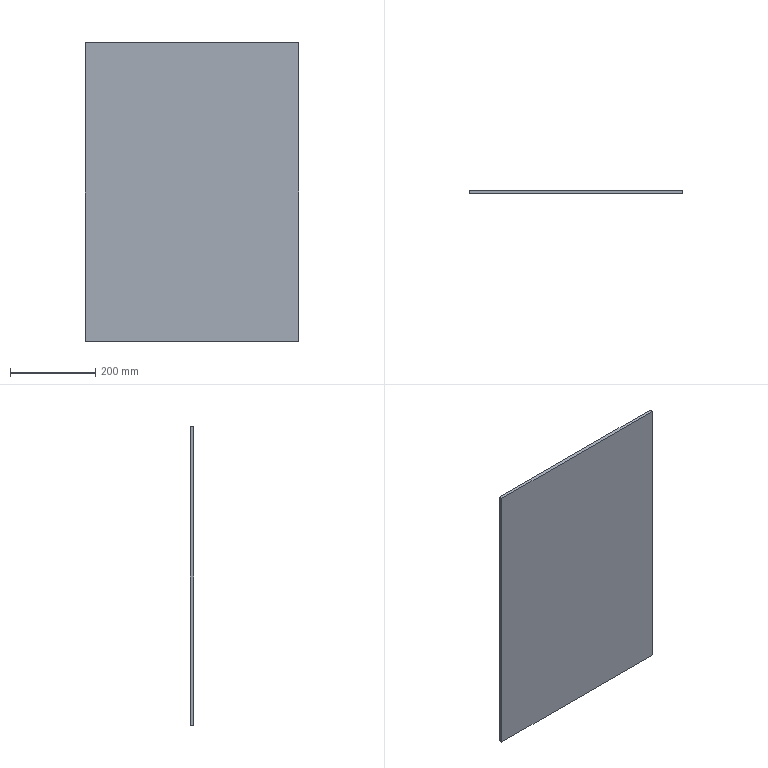Part | SolidWorks | features FlatPattern 1, SMBaseFlange 1, SheetMetal 1 | 1 solid | 6 faces | box 500 x 8 x 700 mm | volume 2800000 mm3 | plane 6
STEP:
#1=CARTESIAN_POINT('',(0.,0.,-700.));
#2=VERTEX_POINT('',#1);
#3=CARTESIAN_POINT('',(0.,0.,0.));
#4=VERTEX_POINT('',#3);
#5=CARTESIAN_POINT('',(0.,0.,0.));
#6=DIRECTION('',(0.,0.,1.));
#7=VECTOR('',#6,1000.);
#8=LINE('',#5,#7);
#9=EDGE_CURVE('',#2,#4,#8,.T.);
#10=ORIENTED_EDGE('',*,*,#9,.F.);
#11=CARTESIAN_POINT('',(0.,-8.,-700.));
#12=VERTEX_POINT('',#11);
#13=CARTESIAN_POINT('',(0.,-8.,-700.));
#14=DIRECTION('',(0.,1.,0.));
#15=VECTOR('',#14,1000.);
#16=LINE('',#13,#15);
#17=EDGE_CURVE('',#12,#2,#16,.T.);
#18=ORIENTED_EDGE('',*,*,#17,.F.);
#19=CARTESIAN_POINT('',(0.,-8.,0.));
#20=VERTEX_POINT('',#19);
#21=CARTESIAN_POINT('',(0.,-8.,0.));
#22=DIRECTION('',(0.,0.,1.));
#23=VECTOR('',#22,1000.);
#24=LINE('',#21,#23);
#25=EDGE_CURVE('',#12,#20,#24,.T.);
#26=ORIENTED_EDGE('',*,*,#25,.T.);
#27=CARTESIAN_POINT('',(0.,-8.,0.));
#28=DIRECTION('',(0.,1.,0.));
#29=VECTOR('',#28,1000.);
#30=LINE('',#27,#29);
#31=EDGE_CURVE('',#20,#4,#30,.T.);
#32=ORIENTED_EDGE('',*,*,#31,.T.);
#33=EDGE_LOOP('',(#10,#18,#26,#32));
#34=FACE_OUTER_BOUND('',#33,.T.);
#35=CARTESIAN_POINT('',(0.,-8.,0.));
#36=DIRECTION('',(-1.,0.,0.));
#37=DIRECTION('',(0.,0.,1.));
#38=AXIS2_PLACEMENT_3D('',#35,#36,#37);
#39=PLANE('',#38);
#40=ADVANCED_FACE('',(#34),#39,.T.);
#41=CARTESIAN_POINT('',(500.,0.,-700.));
#42=VERTEX_POINT('',#41);
#43=CARTESIAN_POINT('',(0.,0.,-700.));
#44=DIRECTION('',(-1.,0.,0.));
#45=VECTOR('',#44,1000.);
#46=LINE('',#43,#45);
#47=EDGE_CURVE('',#42,#2,#46,.T.);
#48=ORIENTED_EDGE('',*,*,#47,.F.);
#49=CARTESIAN_POINT('',(500.,-8.,-700.));
#50=VERTEX_POINT('',#49);
#51=CARTESIAN_POINT('',(500.,-8.,-700.));
#52=DIRECTION('',(0.,1.,0.));
#53=VECTOR('',#52,1000.);
#54=LINE('',#51,#53);
#55=EDGE_CURVE('',#50,#42,#54,.T.);
#56=ORIENTED_EDGE('',*,*,#55,.F.);
#57=CARTESIAN_POINT('',(0.,-8.,-700.));
#58=DIRECTION('',(-1.,0.,0.));
#59=VECTOR('',#58,1000.);
#60=LINE('',#57,#59);
#61=EDGE_CURVE('',#50,#12,#60,.T.);
#62=ORIENTED_EDGE('',*,*,#61,.T.);
#63=ORIENTED_EDGE('',*,*,#17,.T.);
#64=EDGE_LOOP('',(#48,#56,#62,#63));
#65=FACE_OUTER_BOUND('',#64,.T.);
#66=CARTESIAN_POINT('',(0.,-8.,-700.));
#67=DIRECTION('',(0.,0.,-1.));
#68=DIRECTION('',(-1.,0.,0.));
#69=AXIS2_PLACEMENT_3D('',#66,#67,#68);
#70=PLANE('',#69);
#71=ADVANCED_FACE('',(#65),#70,.T.);
#72=CARTESIAN_POINT('',(500.,0.,0.));
#73=VERTEX_POINT('',#72);
#74=CARTESIAN_POINT('',(500.,0.,0.));
#75=DIRECTION('',(0.,0.,-1.));
#76=VECTOR('',#75,1000.);
#77=LINE('',#74,#76);
#78=EDGE_CURVE('',#73,#42,#77,.T.);
#79=ORIENTED_EDGE('',*,*,#78,.F.);
#80=CARTESIAN_POINT('',(500.,-8.,0.));
#81=VERTEX_POINT('',#80);
#82=CARTESIAN_POINT('',(500.,-8.,0.));
#83=DIRECTION('',(0.,1.,0.));
#84=VECTOR('',#83,1000.);
#85=LINE('',#82,#84);
#86=EDGE_CURVE('',#81,#73,#85,.T.);
#87=ORIENTED_EDGE('',*,*,#86,.F.);
#88=CARTESIAN_POINT('',(500.,-8.,0.));
#89=DIRECTION('',(0.,0.,-1.));
#90=VECTOR('',#89,1000.);
#91=LINE('',#88,#90);
#92=EDGE_CURVE('',#81,#50,#91,.T.);
#93=ORIENTED_EDGE('',*,*,#92,.T.);
#94=ORIENTED_EDGE('',*,*,#55,.T.);
#95=EDGE_LOOP('',(#79,#87,#93,#94));
#96=FACE_OUTER_BOUND('',#95,.T.);
#97=CARTESIAN_POINT('',(500.,-8.,0.));
#98=DIRECTION('',(1.,0.,0.));
#99=DIRECTION('',(0.,0.,-1.));
#100=AXIS2_PLACEMENT_3D('',#97,#98,#99);
#101=PLANE('',#100);
#102=ADVANCED_FACE('',(#96),#101,.T.);
#103=CARTESIAN_POINT('',(0.,0.,0.));
#104=DIRECTION('',(1.,0.,0.));
#105=VECTOR('',#104,1000.);
#106=LINE('',#103,#105);
#107=EDGE_CURVE('',#4,#73,#106,.T.);
#108=ORIENTED_EDGE('',*,*,#107,.F.);
#109=ORIENTED_EDGE('',*,*,#31,.F.);
#110=CARTESIAN_POINT('',(0.,-8.,0.));
#111=DIRECTION('',(1.,0.,0.));
#112=VECTOR('',#111,1000.);
#113=LINE('',#110,#112);
#114=EDGE_CURVE('',#20,#81,#113,.T.);
#115=ORIENTED_EDGE('',*,*,#114,.T.);
#116=ORIENTED_EDGE('',*,*,#86,.T.);
#117=EDGE_LOOP('',(#108,#109,#115,#116));
#118=FACE_OUTER_BOUND('',#117,.T.);
#119=CARTESIAN_POINT('',(0.,-8.,0.));
#120=DIRECTION('',(0.,0.,1.));
#121=DIRECTION('',(1.,0.,0.));
#122=AXIS2_PLACEMENT_3D('',#119,#120,#121);
#123=PLANE('',#122);
#124=ADVANCED_FACE('',(#118),#123,.T.);
#125=ORIENTED_EDGE('',*,*,#25,.F.);
#126=ORIENTED_EDGE('',*,*,#61,.F.);
#127=ORIENTED_EDGE('',*,*,#92,.F.);
#128=ORIENTED_EDGE('',*,*,#114,.F.);
#129=EDGE_LOOP('',(#125,#126,#127,#128));
#130=FACE_OUTER_BOUND('',#129,.T.);
#131=CARTESIAN_POINT('',(0.,-8.,-700.));
#132=DIRECTION('',(0.,-1.,0.));
#133=DIRECTION('',(0.,0.,-1.));
#134=AXIS2_PLACEMENT_3D('',#131,#132,#133);
#135=PLANE('',#134);
#136=ADVANCED_FACE('',(#130),#135,.T.);
#137=ORIENTED_EDGE('',*,*,#9,.T.);
#138=ORIENTED_EDGE('',*,*,#107,.T.);
#139=ORIENTED_EDGE('',*,*,#78,.T.);
#140=ORIENTED_EDGE('',*,*,#47,.T.);
#141=EDGE_LOOP('',(#137,#138,#139,#140));
#142=FACE_OUTER_BOUND('',#141,.T.);
#143=CARTESIAN_POINT('',(0.,0.,-700.));
#144=DIRECTION('',(0.,-1.,0.));
#145=DIRECTION('',(0.,0.,-1.));
#146=AXIS2_PLACEMENT_3D('',#143,#144,#145);
#147=PLANE('',#146);
#148=ADVANCED_FACE('',(#142),#147,.F.);
#149=CLOSED_SHELL('',(#40,#71,#102,#124,#136,#148));
#150=MANIFOLD_SOLID_BREP('',#149);
#151=CARTESIAN_POINT('',(0.,0.,0.));
#152=DIRECTION('',(0.,0.,1.));
#153=DIRECTION('',(1.,0.,0.));
#154=AXIS2_PLACEMENT_3D('',#151,#152,#153);
#155=(LENGTH_UNIT()NAMED_UNIT(*)SI_UNIT(.MILLI.,.METRE.));
#156=UNCERTAINTY_MEASURE_WITH_UNIT(LENGTH_MEASURE(0.00001),#155,'','');
#157=(NAMED_UNIT(*)PLANE_ANGLE_UNIT()SI_UNIT($,.RADIAN.));
#158=(NAMED_UNIT(*)SI_UNIT($,.STERADIAN.)SOLID_ANGLE_UNIT());
#159=(GEOMETRIC_REPRESENTATION_CONTEXT(3)GLOBAL_UNCERTAINTY_ASSIGNED_CONTEXT((#156))GLOBAL_UNIT_ASSIGNED_CONTEXT((#155,#157,#158))REPRESENTATION_CONTEXT('',''));
#160=ADVANCED_BREP_SHAPE_REPRESENTATION('',(#150,#154),#159);